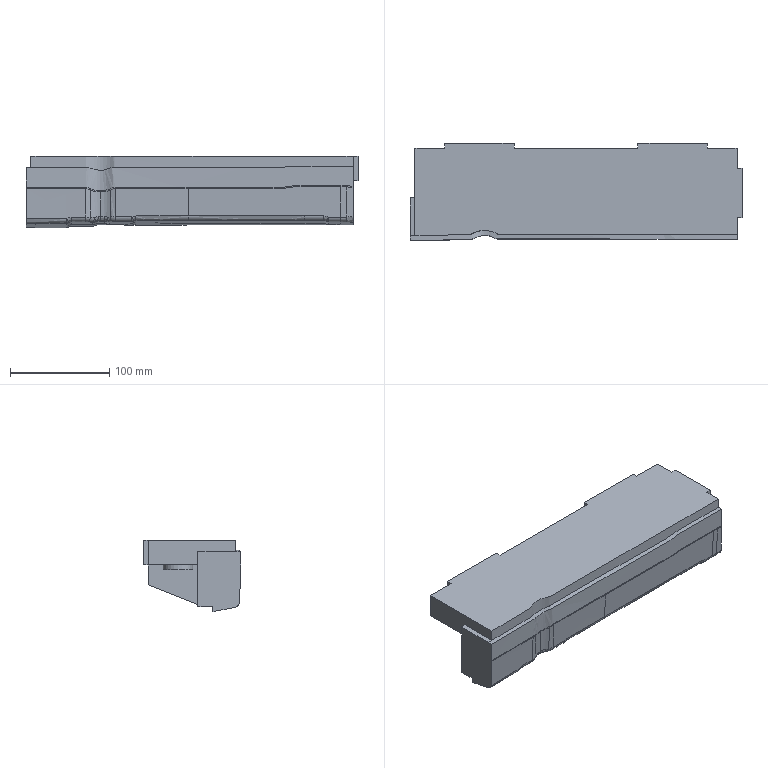Part | NX | features solid 2 | 1 solid | 149 faces | box 335 x 98.257 x 72.256 mm | volume 1449012 mm3 | spline 111 | plane 33 | cylinder 5 | commonest cylinder face diameters 30 x5